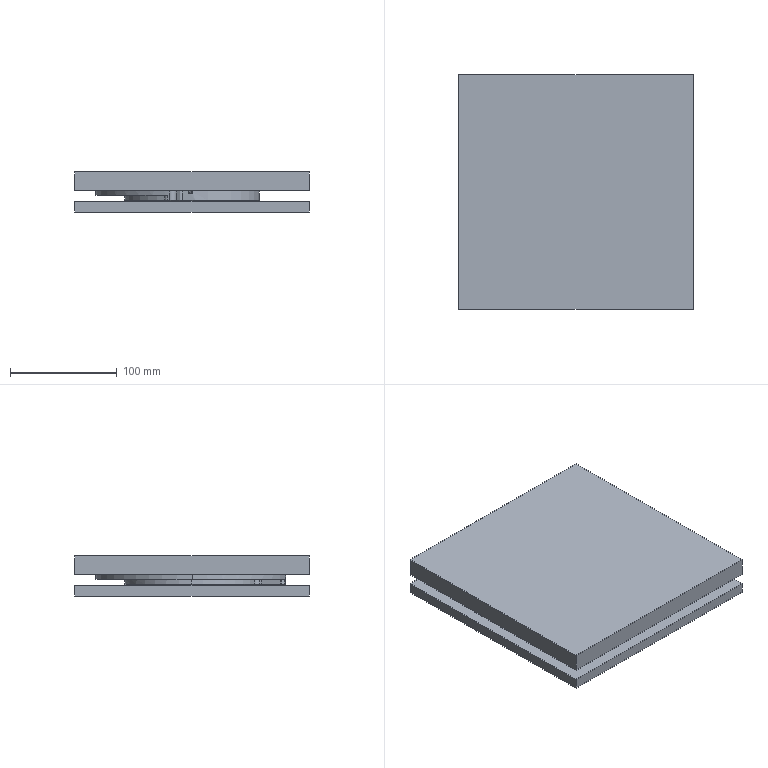NC program | NX | posted with a generic post | part box 220 x 220 x 37.5 mm
Lines 4914 to 5591 of 13716:
(ZLEVEL_PROFILE_COPY_1_COPY , TOOL : D4)
N9766 T10 M6
N9768 G54
N9770 G17 G0 G90 X58.048 Y-36.747 S9500 M3
N9772 G43 Z30. H10
N9774 Z-0.4
N9776 G94 G1 Y-36.054 F1000.
N9778 G3 X57.848 Y-35.708 R0.4
N9780 G1 X55.265 Y-34.217 F1500.
N9782 G2 X53.663 Y-36.678 R65.
N9784 G3 X53.633 Y-37.077 R0.4
N9786 G1 X53.931 Y-37.698
N9788 G0 X58.048 Y-36.747 Z-0.8
N9790 G1 Y-36.055 F1000.
N9792 G3 X57.848 Y-35.708 R0.4
N9794 G1 X55.265 Y-34.217 F1500.
N9796 G2 X53.663 Y-36.678 R65.
N9798 G3 X53.632 Y-37.077 R0.4
N9800 G1 X53.93 Y-37.698
N9802 G0 X58.049 Y-36.748 Z-1.2
N9804 G1 Y-36.055 F1000.
N9806 G3 X57.849 Y-35.708 R0.4
N9808 G1 X55.265 Y-34.217 F1500.
N9810 G2 X53.663 Y-36.679 R65.
N9812 G3 X53.632 Y-37.078 R0.4
N9814 G1 X53.93 Y-37.698
N9816 G0 X58.049 Y-36.748 Z-1.6
N9818 G1 Y-36.055 F1000.
N9820 G3 X57.849 Y-35.709 R0.4
N9822 G1 X55.265 Y-34.217 F1500.
N9824 G2 X53.662 Y-36.679 R65.
N9826 G3 X53.632 Y-37.078 R0.4
N9828 G1 X53.93 Y-37.699
N9830 G0 X58.049 Y-36.748 Z-2.
N9832 G1 Y-36.055 F1000.
N9834 G3 X57.849 Y-35.709 R0.4
N9836 G1 X55.265 Y-34.217 F1500.
N9838 G2 X53.662 Y-36.679 R65.
N9840 G3 X53.632 Y-37.078 R0.4
N9842 G1 X53.93 Y-37.699
N9844 G0 X58.05 Y-36.748 Z-2.4
N9846 G1 Y-36.055 F1000.
N9848 G3 X57.85 Y-35.709 R0.4
N9850 G1 X55.265 Y-34.217 F1500.
N9852 G2 X53.662 Y-36.68 R65.
N9854 G3 X53.632 Y-37.078 R0.4
N9856 G1 X53.93 Y-37.699
N9858 G0 X58.05 Y-36.748 Z-2.8
N9860 G1 Y-36.055 F1000.
N9862 G3 X57.85 Y-35.709 R0.4
N9864 G1 X55.265 Y-34.217 F1500.
N9866 G2 X53.662 Y-36.68 R65.
N9868 G3 X53.631 Y-37.079 R0.4
N9870 G1 X53.929 Y-37.7
N9872 G0 X58.05 Y-36.748 Z-3.2
N9874 G1 Y-36.056 F1000.
N9876 G3 X57.85 Y-35.709 R0.4
N9878 G1 X55.265 Y-34.217 F1500.
N9880 G2 X53.662 Y-36.68 R65.
N9882 G3 X53.631 Y-37.079 R0.4
N9884 G1 X53.929 Y-37.7
N9886 G0 X58.051 Y-36.749 Z-3.6
N9888 G1 Y-36.056 F1000.
N9890 G3 X57.851 Y-35.709 R0.4
N9892 G1 X55.265 Y-34.217 F1500.
N9894 G2 X53.661 Y-36.681 R65.
N9896 G3 X53.631 Y-37.079 R0.4
N9898 G1 X53.929 Y-37.7
N9900 G0 X58.051 Y-36.749 Z-4.
N9902 G1 Y-36.056 F1000.
N9904 G3 X57.851 Y-35.71 R0.4
N9906 G1 X55.265 Y-34.217 F1500.
N9908 G2 X53.661 Y-36.681 R65.
N9910 G3 X53.631 Y-37.08 R0.4
N9912 G1 X53.929 Y-37.701
N9914 G0 X58.051 Y-36.749 Z-4.4
N9916 G1 Y-36.056 F1000.
N9918 G3 X57.851 Y-35.71 R0.4
N9920 G1 X55.265 Y-34.217 F1500.
N9922 G2 X53.661 Y-36.681 R65.
N9924 G3 X53.631 Y-37.08 R0.4
N9926 G1 X53.929 Y-37.701
N9928 G0 X58.052 Y-36.749 Z-4.8
N9930 G1 Y-36.056 F1000.
N9932 G3 X57.852 Y-35.71 R0.4
N9934 G1 X55.265 Y-34.217 F1500.
N9936 G2 X53.661 Y-36.681 R65.
N9938 G3 X53.63 Y-37.08 R0.4
N9940 G1 X53.928 Y-37.701
N9942 G0 X58.052 Y-36.749 Z-5.2
N9944 G1 Y-36.057 F1000.
N9946 G3 X57.852 Y-35.71 R0.4
N9948 G1 X55.265 Y-34.217 F1500.
N9950 G2 X53.66 Y-36.682 R65.
N9952 G3 X53.63 Y-37.081 R0.4
N9954 G1 X53.928 Y-37.701
N9956 G0 X58.052 Y-36.75 Z-5.6
N9958 G1 Y-36.057 F1000.
N9960 G3 X57.852 Y-35.71 R0.4
N9962 G1 X55.265 Y-34.217 F1500.
N9964 G2 X53.66 Y-36.682 R65.
N9966 G3 X53.63 Y-37.081 R0.4
N9968 G1 X53.928 Y-37.702
N9970 G0 X58.053 Y-36.75 Z-6.
N9972 G1 Y-36.057 F1000.
N9974 G3 X57.853 Y-35.711 R0.4
N9976 G1 X55.265 Y-34.217 F1500.
N9978 G2 X53.66 Y-36.682 R65.
N9980 G3 X53.63 Y-37.081 R0.4
N9982 G1 X53.928 Y-37.702
N9984 G0 X58.053 Y-36.75 Z-6.4
N9986 G1 Y-36.057 F1000.
N9988 G3 X57.853 Y-35.711 R0.4
N9990 G1 X55.265 Y-34.217 F1500.
N9992 G2 X53.66 Y-36.683 R65.
N9994 G3 X53.629 Y-37.082 R0.4
N9996 G1 X53.927 Y-37.702
N9998 G0 X58.053 Y-36.75 Z-6.8
N10000 G1 Y-36.057 F1000.
N10002 G3 X57.853 Y-35.711 R0.4
N10004 G1 X55.265 Y-34.217 F1500.
N10006 G2 X53.66 Y-36.683 R65.
N10008 G3 X53.629 Y-37.082 R0.4
N10010 G1 X53.927 Y-37.703
N10012 G0 X58.054 Y-36.75 Z-7.2
N10014 G1 Y-36.058 F1000.
N10016 G3 X57.854 Y-35.711 R0.4
N10018 G1 X55.265 Y-34.217 F1500.
N10020 G2 X53.66 Y-36.683 R65.
N10022 G3 X53.629 Y-37.082 R0.4
N10024 G1 X53.927 Y-37.703
N10026 G0 X58.054 Y-36.751 Z-7.6
N10028 G1 Y-36.058 F1000.
N10030 G3 X57.854 Y-35.712 R0.4
N10032 G1 X55.265 Y-34.217 F1500.
N10034 G2 X53.66 Y-36.683 R65.
N10036 G3 X53.629 Y-37.082 R0.4
N10038 G1 X53.927 Y-37.703
N10040 G0 X58.055 Y-36.751 Z-8.
N10042 G1 Y-36.058 F1000.
N10044 G3 X57.855 Y-35.712 R0.4
N10046 G1 X55.265 Y-34.217 F1500.
N10048 G2 X53.66 Y-36.683 R65.
N10050 G3 X53.629 Y-37.082 R0.4
N10052 G1 X53.927 Y-37.703
N10054 G0 X58.055 Y-36.751 Z-8.4
N10056 G1 Y-36.059 F1000.
N10058 G3 X57.855 Y-35.712 R0.4
N10060 G1 X55.265 Y-34.217 F1500.
N10062 G2 X53.66 Y-36.683 R65.
N10064 G3 X53.629 Y-37.082 R0.4
N10066 G1 X53.927 Y-37.703
N10068 G0 X58.056 Y-36.752 Z-8.8
N10070 G1 Y-36.059 F1000.
N10072 G3 X57.856 Y-35.713 R0.4
N10074 G1 X55.265 Y-34.217 F1500.
N10076 G2 X53.66 Y-36.683 R65.
N10078 G3 X53.629 Y-37.082 R0.4
N10080 G1 X53.927 Y-37.703
N10082 G0 X58.057 Y-36.752 Z-9.2
N10084 G1 Y-36.059 F1000.
N10086 G3 X57.857 Y-35.713 R0.4
N10088 G1 X55.265 Y-34.217 F1500.
N10090 G2 X53.659 Y-36.683 R65.
N10092 G3 X53.629 Y-37.082 R0.4
N10094 G1 X53.927 Y-37.703
N10096 G0 X58.057 Y-36.753 Z-9.6
N10098 G1 Y-36.06 F1000.
N10100 G3 X57.857 Y-35.713 R0.4
N10102 G1 X55.265 Y-34.217 F1500.
N10104 G2 X53.659 Y-36.683 R65.
N10106 G3 X53.629 Y-37.082 R0.4
N10108 G1 X53.927 Y-37.703
N10110 G0 X58.058 Y-36.753 Z-10.
N10112 G1 Y-36.06 F1000.
N10114 G3 X57.858 Y-35.714 R0.4
N10116 G1 X55.265 Y-34.217 F1500.
N10118 G2 X53.659 Y-36.683 R65.
N10120 G3 X53.629 Y-37.082 R0.4
N10122 G1 X53.927 Y-37.703
N10124 G0 X58.056 Y-36.752 Z-10.4
N10126 G1 Y-36.059 F1000.
N10128 G3 X57.856 Y-35.712 R0.4
N10130 G1 X55.265 Y-34.217 F1500.
N10132 G2 X53.66 Y-36.683 R65.
N10134 G3 X53.629 Y-37.082 R0.4
N10136 G1 X53.927 Y-37.703
N10138 G0 X58.056 Y-36.752 Z-10.8
N10140 G1 Y-36.059 F1000.
N10142 G3 X57.856 Y-35.712 R0.4
N10144 G1 X55.265 Y-34.217 F1500.
N10146 G2 X53.66 Y-36.683 R65.
N10148 G3 X53.629 Y-37.082 R0.4
N10150 G1 X53.927 Y-37.703
N10152 G0 X58.056 Y-36.752 Z-11.2
N10154 G1 Y-36.059 F1000.
N10156 G3 X57.856 Y-35.713 R0.4
N10158 G1 X55.265 Y-34.217 F1500.
N10160 G2 X53.66 Y-36.683 R65.
N10162 G3 X53.629 Y-37.082 R0.4
N10164 G1 X53.927 Y-37.703
N10166 G0 X58.056 Y-36.752 Z-11.6
N10168 G1 Y-36.059 F1000.
N10170 G3 X57.856 Y-35.713 R0.4
N10172 G1 X55.265 Y-34.217 F1500.
N10174 G2 X53.659 Y-36.683 R65.
N10176 G3 X53.629 Y-37.082 R0.4
N10178 G1 X53.927 Y-37.703
N10180 G0 X58.057 Y-36.752 Z-12.
N10182 G1 Y-36.059 F1000.
N10184 G3 X57.857 Y-35.713 R0.4
N10186 G1 X55.265 Y-34.217 F1500.
N10188 G2 X53.659 Y-36.683 R65.
N10190 G3 X53.629 Y-37.082 R0.4
N10192 G1 X53.927 Y-37.703
N10194 G0 X55.465 Y-35.402 Z-12.385
N10196 G1 Y-34.563 F1000.
N10198 G3 X55.265 Y-34.217 R0.4
N10200 G2 X53.659 Y-36.683 R65. F1500.
N10202 G3 X53.629 Y-37.082 R0.4
N10204 G1 X53.927 Y-37.703
N10206 G0 X55.465 Y-35.402 Z-12.769
N10208 G1 Y-34.563 F1000.
N10210 G3 X55.265 Y-34.217 R0.4
N10212 G2 X53.659 Y-36.683 R65. F1500.
N10214 G3 X53.629 Y-37.082 R0.4
N10216 G1 X53.927 Y-37.703
N10218 G0 X55.465 Y-35.402 Z-13.154
N10220 G1 Y-34.563 F1000.
N10222 G3 X55.265 Y-34.217 R0.4
N10224 G2 X53.659 Y-36.683 R65. F1500.
N10226 G3 X53.629 Y-37.082 R0.4
N10228 G1 X53.927 Y-37.703
N10230 G0 X55.465 Y-35.402 Z-13.538
N10232 G1 Y-34.563 F1000.
N10234 G3 X55.265 Y-34.217 R0.4
N10236 G2 X53.659 Y-36.683 R65. F1500.
N10238 G3 X53.629 Y-37.082 R0.4
N10240 G1 X53.927 Y-37.703
N10242 G0 X55.465 Y-35.402 Z-13.923
N10244 G1 Y-34.563 F1000.
N10246 G3 X55.265 Y-34.217 R0.4
N10248 G2 X53.659 Y-36.683 R65. F1500.
N10250 G3 X53.629 Y-37.082 R0.4
N10252 G1 X53.927 Y-37.703
N10254 G0 X55.465 Y-35.402 Z-14.308
N10256 G1 Y-34.563 F1000.
N10258 G3 X55.265 Y-34.217 R0.4
N10260 G2 X53.659 Y-36.683 R65. F1500.
N10262 G3 X53.629 Y-37.082 R0.4
N10264 G1 X53.927 Y-37.703
N10266 G0 X55.465 Y-35.402 Z-14.692
N10268 G1 Y-34.563 F1000.
N10270 G3 X55.265 Y-34.217 R0.4
N10272 G2 X53.659 Y-36.683 R65. F1500.
N10274 G3 X53.629 Y-37.082 R0.4
N10276 G1 X53.927 Y-37.703
N10278 G0 X55.465 Y-35.402 Z-15.077
N10280 G1 Y-34.563 F1000.
N10282 G3 X55.265 Y-34.217 R0.4
N10284 G2 X53.659 Y-36.683 R65. F1500.
N10286 G3 X53.629 Y-37.082 R0.4
N10288 G1 X53.927 Y-37.703
N10290 G0 X55.465 Y-35.402 Z-15.462
N10292 G1 Y-34.563 F1000.
N10294 G3 X55.265 Y-34.217 R0.4
N10296 G2 X53.659 Y-36.684 R65. F1500.
N10298 G3 X53.629 Y-37.082 R0.4
N10300 G1 X53.927 Y-37.703
N10302 G0 X55.465 Y-35.402 Z-15.846
N10304 G1 Y-34.563 F1000.
N10306 G3 X55.265 Y-34.217 R0.4
N10308 G2 X53.652 Y-36.694 R65. F1500.
N10310 G3 X53.622 Y-37.093 R0.4
N10312 G1 X53.92 Y-37.713
N10314 G0 X55.465 Y-35.402 Z-16.231
N10316 G1 Y-34.563 F1000.
N10318 G3 X55.265 Y-34.217 R0.4
N10320 G2 X53.659 Y-36.684 R65. F1500.
N10322 G3 X53.629 Y-37.082 R0.4
N10324 G1 X53.927 Y-37.703
N10326 G0 Z30.
N10328 X-65.546 Y5.78
N10330 Z-0.4
N10332 G1 X-64.918 Y6.065 F1000.
N10334 G3 X-64.685 Y6.39 R0.4
N10336 G2 X-64.333 Y9.288 R65. F1500.
N10338 G1 X-64.329 Y9.312
N10340 X-67.284 Y9.833
N10342 G3 X-67.66 Y9.696 R0.4
N10344 G1 X-68.105 Y9.166
N10346 G0 X-65.546 Y5.78 Z-0.8
N10348 G1 X-64.918 Y6.065 F1000.
N10350 G3 X-64.685 Y6.39 R0.4
N10352 G2 X-64.333 Y9.288 R65. F1500.
N10354 G1 X-64.329 Y9.312
N10356 X-67.284 Y9.833
N10358 G3 X-67.66 Y9.696 R0.4
N10360 G1 X-68.105 Y9.166
N10362 G0 X-65.546 Y5.78 Z-1.2
N10364 G1 X-64.918 Y6.065 F1000.
N10366 G3 X-64.685 Y6.39 R0.4
N10368 G2 X-64.333 Y9.288 R65. F1500.
N10370 G1 X-64.329 Y9.312
N10372 X-67.284 Y9.833
N10374 G3 X-67.66 Y9.696 R0.4
N10376 G1 X-68.105 Y9.166
N10378 G0 X-65.546 Y5.78 Z-1.6
N10380 G1 X-64.918 Y6.065 F1000.
N10382 G3 X-64.685 Y6.39 R0.4
N10384 G2 X-64.333 Y9.288 R65. F1500.
N10386 G1 X-64.329 Y9.312
N10388 X-67.284 Y9.833
N10390 G3 X-67.66 Y9.696 R0.4
N10392 G1 X-68.105 Y9.166
N10394 G0 X-65.546 Y5.78 Z-2.
N10396 G1 X-64.918 Y6.065 F1000.
N10398 G3 X-64.685 Y6.39 R0.4
N10400 G2 X-64.333 Y9.288 R65. F1500.
N10402 G1 X-64.329 Y9.312
N10404 X-67.284 Y9.833
N10406 G3 X-67.66 Y9.696 R0.4
N10408 G1 X-68.105 Y9.166
N10410 G0 X-65.546 Y5.78 Z-2.4
N10412 G1 X-64.918 Y6.065 F1000.
N10414 G3 X-64.685 Y6.39 R0.4
N10416 G2 X-64.333 Y9.288 R65. F1500.
N10418 G1 X-64.329 Y9.312
N10420 X-67.284 Y9.833
N10422 G3 X-67.66 Y9.696 R0.4
N10424 G1 X-68.105 Y9.166
N10426 G0 X-65.546 Y5.78 Z-2.8
N10428 G1 X-64.918 Y6.065 F1000.
N10430 G3 X-64.685 Y6.39 R0.4
N10432 G2 X-64.333 Y9.288 R65. F1500.
N10434 G1 X-64.329 Y9.312
N10436 X-67.284 Y9.833
N10438 G3 X-67.66 Y9.696 R0.4
N10440 G1 X-68.105 Y9.166
N10442 G0 X-65.546 Y5.78 Z-3.2
N10444 G1 X-64.918 Y6.065 F1000.
N10446 G3 X-64.685 Y6.39 R0.4
N10448 G2 X-64.333 Y9.288 R65. F1500.
N10450 G1 X-64.329 Y9.312
N10452 X-67.284 Y9.833
N10454 G3 X-67.66 Y9.696 R0.4
N10456 G1 X-68.105 Y9.166
N10458 G0 X-65.546 Y5.78 Z-3.6
N10460 G1 X-64.918 Y6.065 F1000.
N10462 G3 X-64.685 Y6.39 R0.4
N10464 G2 X-64.333 Y9.288 R65. F1500.
N10466 G1 X-64.329 Y9.312
N10468 X-67.284 Y9.833
N10470 G3 X-67.66 Y9.696 R0.4
N10472 G1 X-68.105 Y9.166
N10474 G0 X-65.546 Y5.78 Z-4.
N10476 G1 X-64.918 Y6.065 F1000.
N10478 G3 X-64.685 Y6.39 R0.4
N10480 G2 X-64.333 Y9.288 R65. F1500.
N10482 G1 X-64.329 Y9.312
N10484 X-67.284 Y9.833
N10486 G3 X-67.66 Y9.696 R0.4
N10488 G1 X-68.105 Y9.166
N10490 G0 X-65.546 Y5.78 Z-4.4
N10492 G1 X-64.918 Y6.065 F1000.
N10494 G3 X-64.685 Y6.39 R0.4
N10496 G2 X-64.333 Y9.288 R65. F1500.
N10498 G1 X-64.329 Y9.312
N10500 X-67.284 Y9.833
N10502 G3 X-67.66 Y9.696 R0.4
N10504 G1 X-68.105 Y9.166
N10506 G0 X-65.546 Y5.78 Z-4.8
N10508 G1 X-64.918 Y6.065 F1000.
N10510 G3 X-64.685 Y6.39 R0.4
N10512 G2 X-64.333 Y9.288 R65. F1500.
N10514 G1 X-64.329 Y9.312
N10516 X-67.284 Y9.833
N10518 G3 X-67.66 Y9.696 R0.4
N10520 G1 X-68.105 Y9.166
N10522 G0 X-65.546 Y5.78 Z-5.2
N10524 G1 X-64.918 Y6.065 F1000.
N10526 G3 X-64.685 Y6.39 R0.4
N10528 G2 X-64.333 Y9.288 R65. F1500.
N10530 G1 X-64.329 Y9.312
N10532 X-67.284 Y9.833
N10534 G3 X-67.66 Y9.696 R0.4
N10536 G1 X-68.105 Y9.166
N10538 G0 X-65.546 Y5.78 Z-5.6
N10540 G1 X-64.918 Y6.065 F1000.
N10542 G3 X-64.685 Y6.39 R0.4
N10544 G2 X-64.333 Y9.288 R65. F1500.
N10546 G1 X-64.329 Y9.312
N10548 X-67.284 Y9.833
N10550 G3 X-67.66 Y9.696 R0.4
N10552 G1 X-68.105 Y9.166
N10554 G0 X-65.546 Y5.78 Z-6.
N10556 G1 X-64.918 Y6.065 F1000.
N10558 G3 X-64.685 Y6.39 R0.4
N10560 G2 X-64.333 Y9.288 R65. F1500.
N10562 G1 X-64.329 Y9.312
N10564 X-67.284 Y9.833
N10566 G3 X-67.66 Y9.696 R0.4
N10568 G1 X-68.105 Y9.166
N10570 G0 X-65.546 Y5.78 Z-6.4
N10572 G1 X-64.918 Y6.065 F1000.
N10574 G3 X-64.685 Y6.39 R0.4
N10576 G2 X-64.333 Y9.288 R65. F1500.
N10578 G1 X-64.329 Y9.312
N10580 X-67.284 Y9.833
N10582 G3 X-67.66 Y9.696 R0.4
N10584 G1 X-68.105 Y9.166
N10586 G0 X-65.546 Y5.78 Z-6.8
N10588 G1 X-64.918 Y6.065 F1000.
N10590 G3 X-64.685 Y6.39 R0.4
N10592 G2 X-64.333 Y9.288 R65. F1500.
N10594 G1 X-64.329 Y9.312
N10596 X-67.284 Y9.833
N10598 G3 X-67.66 Y9.696 R0.4
N10600 G1 X-68.105 Y9.166
N10602 G0 X-65.546 Y5.78 Z-7.2
N10604 G1 X-64.918 Y6.065 F1000.
N10606 G3 X-64.685 Y6.39 R0.4
N10608 G2 X-64.333 Y9.288 R65. F1500.
N10610 G1 X-64.329 Y9.312
N10612 X-67.284 Y9.833
N10614 G3 X-67.66 Y9.696 R0.4
N10616 G1 X-68.105 Y9.166
N10618 G0 X-65.546 Y5.78 Z-7.6
N10620 G1 X-64.918 Y6.065 F1000.
N10622 G3 X-64.685 Y6.39 R0.4
N10624 G2 X-64.333 Y9.288 R65. F1500.
N10626 G1 X-64.329 Y9.312
N10628 X-67.284 Y9.833
N10630 G3 X-67.66 Y9.696 R0.4
N10632 G1 X-68.105 Y9.166
N10634 G0 X-65.546 Y5.78 Z-8.
N10636 G1 X-64.918 Y6.065 F1000.
N10638 G3 X-64.685 Y6.39 R0.4
N10640 G2 X-64.333 Y9.288 R65. F1500.
N10642 G1 X-64.329 Y9.312
N10644 X-67.284 Y9.833
N10646 G3 X-67.66 Y9.696 R0.4
N10648 G1 X-68.105 Y9.166
N10650 G0 X-65.546 Y5.78 Z-8.4
N10652 G1 X-64.918 Y6.065 F1000.
N10654 G3 X-64.685 Y6.39 R0.4
N10656 G2 X-64.333 Y9.288 R65. F1500.
N10658 G1 X-64.329 Y9.312
N10660 X-67.284 Y9.833
N10662 G3 X-67.66 Y9.696 R0.4
N10664 G1 X-68.105 Y9.166
N10666 G0 X-65.546 Y5.78 Z-8.8
N10668 G1 X-64.918 Y6.065 F1000.
N10670 G3 X-64.685 Y6.39 R0.4
N10672 G2 X-64.333 Y9.288 R65. F1500.
N10674 G1 X-64.329 Y9.312
N10676 X-67.284 Y9.833
N10678 G3 X-67.66 Y9.696 R0.4
N10680 G1 X-68.105 Y9.166
N10682 G0 X-65.546 Y5.78 Z-9.2
N10684 G1 X-64.918 Y6.065 F1000.
N10686 G3 X-64.685 Y6.39 R0.4
N10688 G2 X-64.333 Y9.288 R65. F1500.
N10690 G1 X-64.329 Y9.312
N10692 X-67.284 Y9.833
N10694 G3 X-67.66 Y9.696 R0.4
N10696 G1 X-68.105 Y9.166
N10698 G0 X-65.546 Y5.78 Z-9.6
N10700 G1 X-64.918 Y6.065 F1000.
N10702 G3 X-64.685 Y6.39 R0.4
N10704 G2 X-64.333 Y9.288 R65. F1500.
N10706 G1 X-64.329 Y9.312
N10708 X-67.284 Y9.833
N10710 G3 X-67.66 Y9.696 R0.4
N10712 G1 X-68.105 Y9.166
N10714 G0 X-65.546 Y5.78 Z-10.
N10716 G1 X-64.918 Y6.065 F1000.
N10718 G3 X-64.685 Y6.39 R0.4
N10720 G2 X-64.333 Y9.288 R65. F1500.
N10722 G1 X-64.329 Y9.312
N10724 X-67.284 Y9.833
N10726 G3 X-67.66 Y9.696 R0.4
N10728 G1 X-68.105 Y9.166
N10730 G0 X-65.546 Y5.78 Z-10.4
N10732 G1 X-64.918 Y6.065 F1000.
N10734 G3 X-64.685 Y6.39 R0.4
N10736 G2 X-64.333 Y9.288 R65. F1500.
N10738 G1 X-64.329 Y9.312
N10740 X-67.284 Y9.833
N10742 G3 X-67.66 Y9.696 R0.4
N10744 G1 X-68.105 Y9.166
N10746 G0 X-65.546 Y5.78 Z-10.8
N10748 G1 X-64.918 Y6.065 F1000.
N10750 G3 X-64.685 Y6.39 R0.4
N10752 G2 X-64.333 Y9.288 R65. F1500.
N10754 G1 X-64.329 Y9.312
N10756 X-67.284 Y9.833
N10758 G3 X-67.66 Y9.696 R0.4
N10760 G1 X-68.105 Y9.166
N10762 G0 X-65.546 Y5.78 Z-11.2
N10764 G1 X-64.918 Y6.065 F1000.
N10766 G3 X-64.685 Y6.39 R0.4
N10768 G2 X-64.333 Y9.288 R65. F1500.
N10770 G1 X-64.329 Y9.312
N10772 X-67.284 Y9.833
N10774 G3 X-67.66 Y9.696 R0.4
N10776 G1 X-68.105 Y9.166
N10778 G0 X-65.546 Y5.78 Z-11.6
N10780 G1 X-64.918 Y6.065 F1000.
N10782 G3 X-64.685 Y6.39 R0.4
N10784 G2 X-64.333 Y9.288 R65. F1500.
N10786 G1 X-64.329 Y9.312
N10788 X-67.284 Y9.833
N10790 G3 X-67.66 Y9.696 R0.4
N10792 G1 X-68.105 Y9.166
N10794 G0 X-65.546 Y5.78 Z-12.
N10796 G1 X-64.918 Y6.065 F1000.
N10798 G3 X-64.685 Y6.39 R0.4
N10800 G2 X-64.333 Y9.288 R65. F1500.
N10802 G1 X-64.329 Y9.312
N10804 X-67.284 Y9.833
N10806 G3 X-67.66 Y9.696 R0.4
N10808 G1 X-68.105 Y9.166
N10810 G0 X-65.546 Y5.78 Z-12.385
N10812 G1 X-64.918 Y6.065 F1000.
N10814 G3 X-64.685 Y6.39 R0.4
N10816 G2 X-64.333 Y9.288 R65. F1500.
N10818 G1 X-64.329 Y9.312
N10820 X-67.284 Y9.833
N10822 G3 X-67.66 Y9.696 R0.4
N10824 G1 X-68.105 Y9.166
N10826 G0 X-65.546 Y5.78 Z-12.769
N10828 G1 X-64.918 Y6.065 F1000.
N10830 G3 X-64.685 Y6.39 R0.4
N10832 G2 X-64.333 Y9.288 R65. F1500.
N10834 G1 X-64.329 Y9.312
N10836 X-67.284 Y9.833
N10838 G3 X-67.66 Y9.696 R0.4
N10840 G1 X-68.105 Y9.166
N10842 G0 X-65.546 Y5.78 Z-13.154
N10844 G1 X-64.918 Y6.065 F1000.
N10846 G3 X-64.685 Y6.39 R0.4
N10848 G2 X-64.333 Y9.288 R65. F1500.
N10850 G1 X-64.329 Y9.312
N10852 X-67.284 Y9.833
N10854 G3 X-67.66 Y9.696 R0.4
N10856 G1 X-68.105 Y9.166
N10858 G0 X-65.546 Y5.78 Z-13.538
N10860 G1 X-64.918 Y6.065 F1000.
N10862 G3 X-64.685 Y6.39 R0.4
N10864 G2 X-64.333 Y9.288 R65. F1500.
N10866 G1 X-64.329 Y9.312
N10868 X-67.284 Y9.833
N10870 G3 X-67.66 Y9.696 R0.4
N10872 G1 X-68.105 Y9.166
N10874 G0 X-65.546 Y5.78 Z-13.923
N10876 G1 X-64.918 Y6.065 F1000.
N10878 G3 X-64.685 Y6.39 R0.4
N10880 G2 X-64.333 Y9.288 R65. F1500.
N10882 G1 X-64.329 Y9.312
N10884 X-67.284 Y9.833
N10886 G3 X-67.66 Y9.696 R0.4
N10888 G1 X-68.105 Y9.166
N10890 G0 X-65.546 Y5.78 Z-14.308
N10892 G1 X-64.918 Y6.065 F1000.
N10894 G3 X-64.685 Y6.39 R0.4
N10896 G2 X-64.333 Y9.288 R65. F1500.
N10898 G1 X-64.329 Y9.312
N10900 X-67.284 Y9.833
N10902 G3 X-67.66 Y9.696 R0.4
N10904 G1 X-68.105 Y9.166
N10906 G0 X-65.546 Y5.78 Z-14.692
N10908 G1 X-64.918 Y6.065 F1000.
N10910 G3 X-64.685 Y6.39 R0.4
N10912 G2 X-64.333 Y9.288 R65. F1500.
N10914 G1 X-64.329 Y9.312
N10916 X-67.284 Y9.833
N10918 G3 X-67.66 Y9.696 R0.4
N10920 G1 X-68.105 Y9.166
N10922 G0 X-65.546 Y5.78 Z-15.077
N10924 G1 X-64.918 Y6.065 F1000.
N10926 G3 X-64.685 Y6.39 R0.4
N10928 G2 X-64.333 Y9.288 R65. F1500.
N10930 G1 X-64.329 Y9.312
N10932 X-67.284 Y9.833
N10934 G3 X-67.66 Y9.696 R0.4
N10936 G1 X-68.105 Y9.166
N10938 G0 X-65.546 Y5.78 Z-15.462
N10940 G1 X-64.918 Y6.065 F1000.
N10942 G3 X-64.685 Y6.39 R0.4
N10944 G2 X-64.333 Y9.288 R65. F1500.
N10946 G1 X-64.329 Y9.312
N10948 X-67.284 Y9.833
N10950 G3 X-67.66 Y9.696 R0.4
N10952 G1 X-68.105 Y9.166
N10954 G0 X-65.546 Y5.78 Z-15.846
N10956 G1 X-64.918 Y6.065 F1000.
N10958 G3 X-64.685 Y6.39 R0.4
N10960 G2 X-64.333 Y9.288 R65. F1500.
N10962 G1 X-64.329 Y9.312
N10964 X-67.284 Y9.833
N10966 G3 X-67.66 Y9.696 R0.4
N10968 G1 X-68.105 Y9.166
N10970 G0 X-65.546 Y5.78 Z-16.231
N10972 G1 X-64.918 Y6.065 F1000.
N10974 G3 X-64.685 Y6.39 R0.4
N10976 G2 X-64.333 Y9.288 R65. F1500.
N10978 G1 X-64.329 Y9.312
N10980 X-67.284 Y9.833
N10982 G3 X-67.66 Y9.696 R0.4
N10984 G1 X-68.105 Y9.166
N10986 G0 Z30.
N10988 M5
(ZLEVEL_PROFILE_COPY_1_COPY_COPY_COPY_COPY_2_COPY , TOOL : D6A45)
N10990 T18 M6
N10992 G54
N10994 G17 G0 G90 X37.19 Y41.08 S7000 M3
N10996 G43 Z30. H18
N10998 Z-1.
N11000 G94 G1 X36.52 Y42.241 F1000.
N11002 G3 X36. Y42.541 R0.6
N11004 G1 X35.996
N11006 G3 X31.959 Y38.496 R4.041
N11008 X36. Y42.541 R-4.041
N11010 X35.48 Y42.241 R0.6
N11012 G1 X34.81 Y41.08
N11014 G0 Z30.
N11016 X53.887 Y17.038
N11018 Z-1.
N11020 G1 X52.86 Y17.9
N11022 G3 X52.269 Y18.004 R0.6
N11024 G1 X38.094 Y12.845
N11026 G3 X35.537 Y8.145 R4.041
N11028 G2 X35.897 Y6.373 R36.459
N11030 G3 X38.106 Y4.699 R2.041
N11032 G1 X42.655 Y5.145
N11034 G2 X45.898 Y2.352 R2.959
N11036 X44.998 Y-9.348 R45.959
N11038 X41.365 Y-11.611 R2.959
N11040 G1 X36.938 Y-10.475
N11042 G3 X34.499 Y-11.792 R2.041
N11044 G2 X-31.927 Y-17.603 R36.459
N11046 G3 X-34.558 Y-16.73 R2.041
N11048 G1 X-38.721 Y-18.618
N11050 G2 X-42.691 Y-17.019 R2.959
N11052 X-45.929 Y-1.658 R45.959
N11054 X-42.941 Y1.407 R2.959
N11056 G1 X-38.353 Y1.36
N11058 G3 X-36.316 Y3.221 R2.041
N11060 G2 X-35.537 Y8.145 R36.459
N11062 G3 X-38.094 Y12.845 R4.041
N11064 G1 X-52.269 Y18.004
N11066 G3 X-57.558 Y15.241 R4.041
N11068 X57.558 Y15.241 R-59.541
N11070 X52.269 Y18.004 R4.041
N11072 X51.883 Y17.545 R0.6
N11074 G1 X51.703 Y16.521
N11076 G0 Z30.
N11078 X73.305 Y-44.735
N11080 Z-1.
N11082 G1 Y-43.776
N11084 G3 X73.005 Y-43.257 R0.6
N11086 G1 X55.786 Y-33.315
N11088 G3 X54.38 Y-33.668 R1.041
N11090 G2 X-63.299 Y9.163 R63.959
N11092 G3 X-64.149 Y10.338 R1.041
N11094 G1 X-83.73 Y13.791
N11096 G2 X-88.492 Y21.037 R5.959
N11098 X81.311 Y-40.767 R-90.959
N11100 X73.005 Y-43.257 R5.959
N11102 G3 X72.405 Y-43.257 R0.6
N11104 G1 X71.505 Y-43.776
N11106 G0 Z30.
N11108 M5